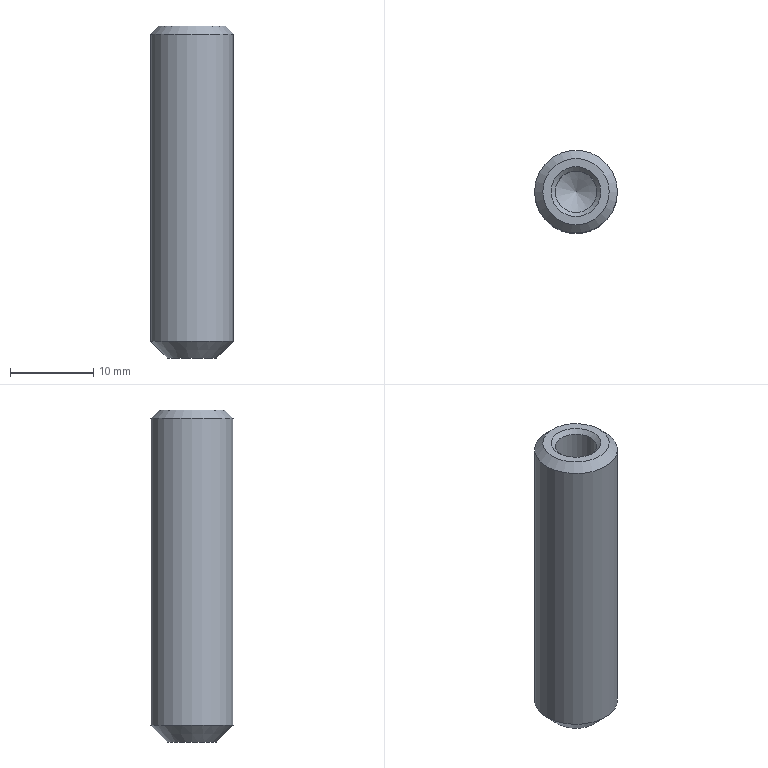Part | STEP file | 冲床-300配套压波_id62_x_t | 1 solid | 8 faces | box 10 x 10 x 40 mm | volume 2825 mm3 | cone 4 | cylinder 2 | plane 2 | commonest cylinder face diameters 5 x1 10 x1
STEP:
#1=CARTESIAN_POINT('',(1215.,-117.5,23.));
#2=VERTEX_POINT('',#1);
#3=CARTESIAN_POINT('',(1220.,-117.5,23.));
#4=DIRECTION('',(0.,0.,-1.));
#5=DIRECTION('',(-1.,0.,0.));
#6=AXIS2_PLACEMENT_3D('',#3,#4,#5);
#7=CIRCLE('',#6,5.);
#8=EDGE_CURVE('',#2,#2,#7,.T.);
#9=ORIENTED_EDGE('',*,*,#8,.T.);
#10=EDGE_LOOP('',(#9));
#11=FACE_BOUND('',#10,.T.);
#12=CARTESIAN_POINT('',(1215.,-117.5,-14.));
#13=VERTEX_POINT('',#12);
#14=CARTESIAN_POINT('',(1220.,-117.5,-14.));
#15=DIRECTION('',(0.,0.,1.));
#16=DIRECTION('',(-1.,0.,0.));
#17=AXIS2_PLACEMENT_3D('',#14,#15,#16);
#18=CIRCLE('',#17,5.);
#19=EDGE_CURVE('',#13,#13,#18,.T.);
#20=ORIENTED_EDGE('',*,*,#19,.T.);
#21=EDGE_LOOP('',(#20));
#22=FACE_BOUND('',#21,.T.);
#23=CARTESIAN_POINT('',(1220.,-117.5,-16.));
#24=DIRECTION('',(0.,0.,1.));
#25=DIRECTION('',(1.,0.,0.));
#26=AXIS2_PLACEMENT_3D('',#23,#24,#25);
#27=CYLINDRICAL_SURFACE('',#26,5.);
#28=ADVANCED_FACE('',(#11,#22),#27,.T.);
#29=CARTESIAN_POINT('',(1217.,-117.5,-16.));
#30=VERTEX_POINT('',#29);
#31=CARTESIAN_POINT('',(1220.,-117.5,-16.));
#32=DIRECTION('',(0.,0.,-1.));
#33=DIRECTION('',(-1.,0.,0.));
#34=AXIS2_PLACEMENT_3D('',#31,#32,#33);
#35=CIRCLE('',#34,3.);
#36=EDGE_CURVE('',#30,#30,#35,.T.);
#37=ORIENTED_EDGE('',*,*,#36,.T.);
#38=EDGE_LOOP('',(#37));
#39=FACE_OUTER_BOUND('',#38,.T.);
#40=CARTESIAN_POINT('',(1220.,-117.5,-16.));
#41=DIRECTION('',(0.,0.,-1.));
#42=DIRECTION('',(-1.,0.,0.));
#43=AXIS2_PLACEMENT_3D('',#40,#41,#42);
#44=PLANE('',#43);
#45=ADVANCED_FACE('',(#39),#44,.T.);
#46=CARTESIAN_POINT('',(1217.,-117.5,24.));
#47=VERTEX_POINT('',#46);
#48=CARTESIAN_POINT('',(1220.,-117.5,24.));
#49=DIRECTION('',(0.,0.,-1.));
#50=DIRECTION('',(-1.,0.,0.));
#51=AXIS2_PLACEMENT_3D('',#48,#49,#50);
#52=CIRCLE('',#51,3.);
#53=EDGE_CURVE('',#47,#47,#52,.T.);
#54=ORIENTED_EDGE('',*,*,#53,.T.);
#55=EDGE_LOOP('',(#54));
#56=FACE_BOUND('',#55,.T.);
#57=CARTESIAN_POINT('',(1216.,-117.5,24.));
#58=VERTEX_POINT('',#57);
#59=CARTESIAN_POINT('',(1220.,-117.5,24.));
#60=DIRECTION('',(0.,0.,1.));
#61=DIRECTION('',(-1.,0.,0.));
#62=AXIS2_PLACEMENT_3D('',#59,#60,#61);
#63=CIRCLE('',#62,4.);
#64=EDGE_CURVE('',#58,#58,#63,.T.);
#65=ORIENTED_EDGE('',*,*,#64,.T.);
#66=EDGE_LOOP('',(#65));
#67=FACE_BOUND('',#66,.T.);
#68=CARTESIAN_POINT('',(1220.,-117.5,24.));
#69=DIRECTION('',(0.,0.,-1.));
#70=DIRECTION('',(-1.,0.,0.));
#71=AXIS2_PLACEMENT_3D('',#68,#69,#70);
#72=PLANE('',#71);
#73=ADVANCED_FACE('',(#56,#67),#72,.F.);
#74=ORIENTED_EDGE('',*,*,#19,.F.);
#75=EDGE_LOOP('',(#74));
#76=FACE_BOUND('',#75,.T.);
#77=ORIENTED_EDGE('',*,*,#36,.F.);
#78=EDGE_LOOP('',(#77));
#79=FACE_BOUND('',#78,.T.);
#80=CARTESIAN_POINT('',(1220.,-117.5,-16.));
#81=DIRECTION('',(0.,0.,1.));
#82=DIRECTION('',(1.,0.,0.));
#83=AXIS2_PLACEMENT_3D('',#80,#81,#82);
#84=CONICAL_SURFACE('',#83,3.,45.);
#85=ADVANCED_FACE('',(#76,#79),#84,.T.);
#86=ORIENTED_EDGE('',*,*,#64,.F.);
#87=EDGE_LOOP('',(#86));
#88=FACE_BOUND('',#87,.T.);
#89=ORIENTED_EDGE('',*,*,#8,.F.);
#90=EDGE_LOOP('',(#89));
#91=FACE_BOUND('',#90,.T.);
#92=CARTESIAN_POINT('',(1220.,-117.5,23.));
#93=DIRECTION('',(0.,0.,-1.));
#94=DIRECTION('',(-1.,0.,0.));
#95=AXIS2_PLACEMENT_3D('',#92,#93,#94);
#96=CONICAL_SURFACE('',#95,5.,45.);
#97=ADVANCED_FACE('',(#88,#91),#96,.T.);
#98=CARTESIAN_POINT('',(1217.5,-117.5,12.));
#99=VERTEX_POINT('',#98);
#100=CARTESIAN_POINT('',(1220.,-117.5,12.));
#101=DIRECTION('',(0.,0.,1.));
#102=DIRECTION('',(-1.,0.,0.));
#103=AXIS2_PLACEMENT_3D('',#100,#101,#102);
#104=CIRCLE('',#103,2.5);
#105=EDGE_CURVE('',#99,#99,#104,.T.);
#106=ORIENTED_EDGE('',*,*,#105,.T.);
#107=EDGE_LOOP('',(#106));
#108=FACE_BOUND('',#107,.T.);
#109=CARTESIAN_POINT('',(1220.,-117.5,10.498));
#110=VERTEX_POINT('',#109);
#111=VERTEX_LOOP('',#110);
#112=FACE_BOUND('',#111,.T.);
#113=CARTESIAN_POINT('',(1220.,-117.5,12.));
#114=DIRECTION('',(0.,0.,1.));
#115=DIRECTION('',(1.,0.,0.));
#116=AXIS2_PLACEMENT_3D('',#113,#114,#115);
#117=CONICAL_SURFACE('',#116,2.5,59.);
#118=ADVANCED_FACE('',(#108,#112),#117,.F.);
#119=CARTESIAN_POINT('',(1217.5,-117.5,23.5));
#120=VERTEX_POINT('',#119);
#121=CARTESIAN_POINT('',(1220.,-117.5,23.5));
#122=DIRECTION('',(0.,0.,1.));
#123=DIRECTION('',(-1.,0.,0.));
#124=AXIS2_PLACEMENT_3D('',#121,#122,#123);
#125=CIRCLE('',#124,2.5);
#126=EDGE_CURVE('',#120,#120,#125,.T.);
#127=ORIENTED_EDGE('',*,*,#126,.T.);
#128=EDGE_LOOP('',(#127));
#129=FACE_BOUND('',#128,.T.);
#130=ORIENTED_EDGE('',*,*,#105,.F.);
#131=EDGE_LOOP('',(#130));
#132=FACE_BOUND('',#131,.T.);
#133=CARTESIAN_POINT('',(1220.,-117.5,24.));
#134=DIRECTION('',(0.,0.,-1.));
#135=DIRECTION('',(-1.,0.,0.));
#136=AXIS2_PLACEMENT_3D('',#133,#134,#135);
#137=CYLINDRICAL_SURFACE('',#136,2.5);
#138=ADVANCED_FACE('',(#129,#132),#137,.F.);
#139=ORIENTED_EDGE('',*,*,#126,.F.);
#140=EDGE_LOOP('',(#139));
#141=FACE_BOUND('',#140,.T.);
#142=ORIENTED_EDGE('',*,*,#53,.F.);
#143=EDGE_LOOP('',(#142));
#144=FACE_BOUND('',#143,.T.);
#145=CARTESIAN_POINT('',(1220.,-117.5,24.));
#146=DIRECTION('',(0.,0.,1.));
#147=DIRECTION('',(1.,0.,0.));
#148=AXIS2_PLACEMENT_3D('',#145,#146,#147);
#149=CONICAL_SURFACE('',#148,3.,45.);
#150=ADVANCED_FACE('',(#141,#144),#149,.F.);
#151=CLOSED_SHELL('',(#28,#45,#73,#85,#97,#118,#138,#150));
#152=MANIFOLD_SOLID_BREP('',#151);
#153=(LENGTH_UNIT()NAMED_UNIT(*)SI_UNIT(.MILLI.,.METRE.));
#154=UNCERTAINTY_MEASURE_WITH_UNIT(LENGTH_MEASURE(0.00002),#153,'','');
#155=(NAMED_UNIT(*)PLANE_ANGLE_UNIT()SI_UNIT($,.RADIAN.));
#156=PLANE_ANGLE_MEASURE_WITH_UNIT(PLANE_ANGLE_MEASURE(0.01745),#155);
#157=DIMENSIONAL_EXPONENTS(0.,0.,0.,0.,0.,0.,0.);
#158=(CONVERSION_BASED_UNIT('DEGREE',#156)NAMED_UNIT(#157)PLANE_ANGLE_UNIT());
#159=(NAMED_UNIT(*)SI_UNIT($,.STERADIAN.)SOLID_ANGLE_UNIT());
#160=(GEOMETRIC_REPRESENTATION_CONTEXT(3)GLOBAL_UNCERTAINTY_ASSIGNED_CONTEXT((#154))GLOBAL_UNIT_ASSIGNED_CONTEXT((#153,#158,#159))REPRESENTATION_CONTEXT('',''));
#161=ADVANCED_BREP_SHAPE_REPRESENTATION('',(#152),#160);